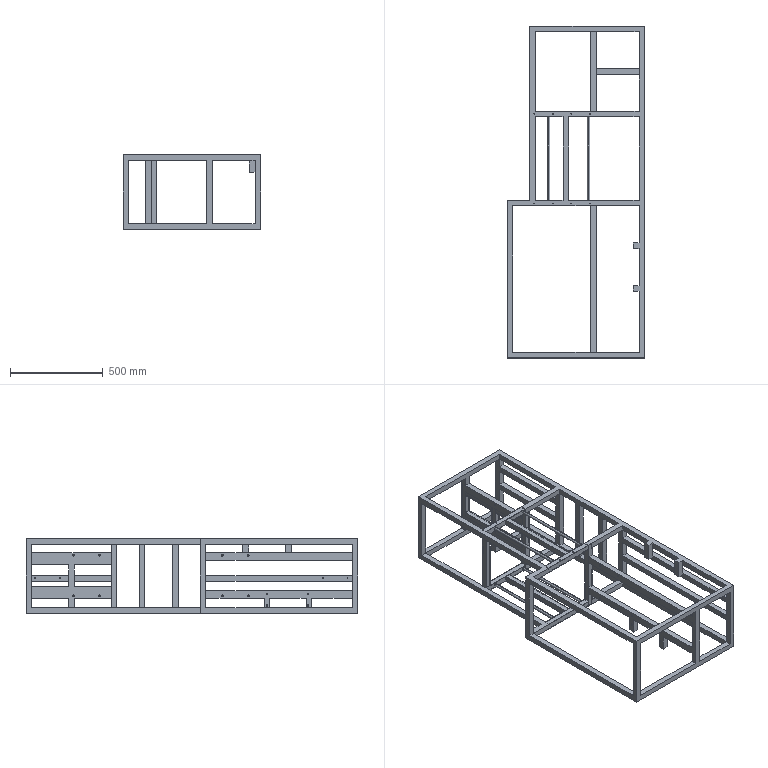Part | STEP file | Frame | 1 solid | 360 faces | box 740 x 1790 x 402.356 mm | volume 20261425 mm3 | plane 231 | cylinder 80 | cone 49 | commonest cylinder face diameters 4.2 x32 8.5 x24 5 x16 15 x8